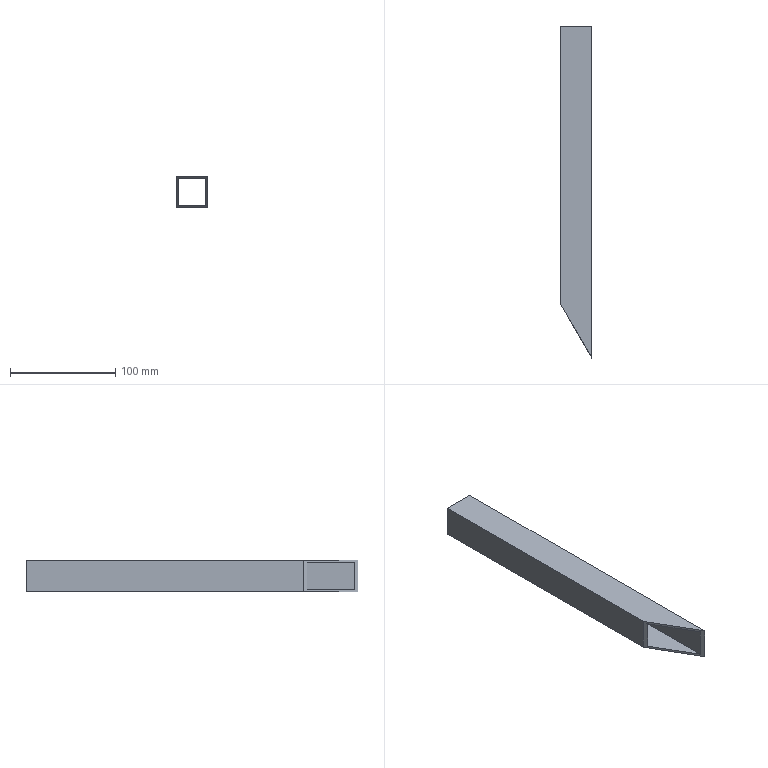Part | NX | features solid 2 | 1 solid | 10 faces | box 30 x 315 x 30 mm | volume 64740 mm3 | plane 10
STEP:
#1=CARTESIAN_POINT('',(-115.,435.,-75.));
#2=VERTEX_POINT('',#1);
#3=CARTESIAN_POINT('',(-115.,750.,-75.));
#4=VERTEX_POINT('',#3);
#5=CARTESIAN_POINT('',(-115.,615.,-75.));
#6=DIRECTION('',(0.,-1.,0.));
#7=VECTOR('',#6,1000.);
#8=LINE('',#5,#7);
#9=EDGE_CURVE('',#2,#4,#8,.F.);
#10=ORIENTED_EDGE('',*,*,#9,.F.);
#11=CARTESIAN_POINT('',(-145.,486.962,-75.));
#12=VERTEX_POINT('',#11);
#13=CARTESIAN_POINT('',(-196.692,576.495,-75.));
#14=DIRECTION('',(0.5,-0.866,0.));
#15=VECTOR('',#14,1000.);
#16=LINE('',#13,#15);
#17=EDGE_CURVE('',#2,#12,#16,.F.);
#18=ORIENTED_EDGE('',*,*,#17,.T.);
#19=CARTESIAN_POINT('',(-145.,750.,-75.));
#20=VERTEX_POINT('',#19);
#21=CARTESIAN_POINT('',(-145.,615.,-75.));
#22=DIRECTION('',(0.,-1.,0.));
#23=VECTOR('',#22,1000.);
#24=LINE('',#21,#23);
#25=EDGE_CURVE('',#12,#20,#24,.F.);
#26=ORIENTED_EDGE('',*,*,#25,.T.);
#27=CARTESIAN_POINT('',(-130.,750.,-75.));
#28=DIRECTION('',(-1.,0.,0.));
#29=VECTOR('',#28,1000.);
#30=LINE('',#27,#29);
#31=EDGE_CURVE('',#20,#4,#30,.F.);
#32=ORIENTED_EDGE('',*,*,#31,.T.);
#33=EDGE_LOOP('',(#10,#18,#26,#32));
#34=FACE_BOUND('',#33,.T.);
#35=CARTESIAN_POINT('',(-130.,615.,-75.));
#36=DIRECTION('',(0.,0.,1.));
#37=DIRECTION('',(0.,1.,0.));
#38=AXIS2_PLACEMENT_3D('',#35,#36,#37);
#39=PLANE('',#38);
#40=ADVANCED_FACE('',(#34),#39,.F.);
#41=CARTESIAN_POINT('',(-115.,435.,-45.));
#42=VERTEX_POINT('',#41);
#43=CARTESIAN_POINT('',(-145.,486.962,-45.));
#44=VERTEX_POINT('',#43);
#45=CARTESIAN_POINT('',(-196.692,576.495,-45.));
#46=DIRECTION('',(0.5,-0.866,0.));
#47=VECTOR('',#46,1000.);
#48=LINE('',#45,#47);
#49=EDGE_CURVE('',#42,#44,#48,.F.);
#50=ORIENTED_EDGE('',*,*,#49,.F.);
#51=CARTESIAN_POINT('',(-115.,750.,-45.));
#52=VERTEX_POINT('',#51);
#53=CARTESIAN_POINT('',(-115.,615.,-45.));
#54=DIRECTION('',(0.,-1.,0.));
#55=VECTOR('',#54,1000.);
#56=LINE('',#53,#55);
#57=EDGE_CURVE('',#42,#52,#56,.F.);
#58=ORIENTED_EDGE('',*,*,#57,.T.);
#59=CARTESIAN_POINT('',(-145.,750.,-45.));
#60=VERTEX_POINT('',#59);
#61=CARTESIAN_POINT('',(-130.,750.,-45.));
#62=DIRECTION('',(-1.,0.,0.));
#63=VECTOR('',#62,1000.);
#64=LINE('',#61,#63);
#65=EDGE_CURVE('',#60,#52,#64,.F.);
#66=ORIENTED_EDGE('',*,*,#65,.F.);
#67=CARTESIAN_POINT('',(-145.,615.,-45.));
#68=DIRECTION('',(0.,-1.,0.));
#69=VECTOR('',#68,1000.);
#70=LINE('',#67,#69);
#71=EDGE_CURVE('',#44,#60,#70,.F.);
#72=ORIENTED_EDGE('',*,*,#71,.F.);
#73=EDGE_LOOP('',(#50,#58,#66,#72));
#74=FACE_BOUND('',#73,.T.);
#75=CARTESIAN_POINT('',(-130.,615.,-45.));
#76=DIRECTION('',(0.,0.,1.));
#77=DIRECTION('',(0.,1.,0.));
#78=AXIS2_PLACEMENT_3D('',#75,#76,#77);
#79=PLANE('',#78);
#80=ADVANCED_FACE('',(#74),#79,.T.);
#81=ORIENTED_EDGE('',*,*,#57,.F.);
#82=CARTESIAN_POINT('',(-115.,435.,-75.));
#83=DIRECTION('',(0.,0.,-1.));
#84=VECTOR('',#83,1000.);
#85=LINE('',#82,#84);
#86=EDGE_CURVE('',#42,#2,#85,.T.);
#87=ORIENTED_EDGE('',*,*,#86,.T.);
#88=ORIENTED_EDGE('',*,*,#9,.T.);
#89=CARTESIAN_POINT('',(-115.,750.,-75.));
#90=DIRECTION('',(0.,0.,1.));
#91=VECTOR('',#90,1000.);
#92=LINE('',#89,#91);
#93=EDGE_CURVE('',#4,#52,#92,.T.);
#94=ORIENTED_EDGE('',*,*,#93,.T.);
#95=EDGE_LOOP('',(#81,#87,#88,#94));
#96=FACE_BOUND('',#95,.T.);
#97=CARTESIAN_POINT('',(-115.,615.,-75.));
#98=DIRECTION('',(1.,0.,0.));
#99=DIRECTION('',(0.,0.,-1.));
#100=AXIS2_PLACEMENT_3D('',#97,#98,#99);
#101=PLANE('',#100);
#102=ADVANCED_FACE('',(#96),#101,.T.);
#103=CARTESIAN_POINT('',(-145.,486.962,-75.));
#104=DIRECTION('',(0.,0.,-1.));
#105=VECTOR('',#104,1000.);
#106=LINE('',#103,#105);
#107=EDGE_CURVE('',#44,#12,#106,.T.);
#108=ORIENTED_EDGE('',*,*,#107,.F.);
#109=ORIENTED_EDGE('',*,*,#71,.T.);
#110=CARTESIAN_POINT('',(-145.,750.,-75.));
#111=DIRECTION('',(0.,0.,1.));
#112=VECTOR('',#111,1000.);
#113=LINE('',#110,#112);
#114=EDGE_CURVE('',#20,#60,#113,.T.);
#115=ORIENTED_EDGE('',*,*,#114,.F.);
#116=ORIENTED_EDGE('',*,*,#25,.F.);
#117=EDGE_LOOP('',(#108,#109,#115,#116));
#118=FACE_BOUND('',#117,.T.);
#119=CARTESIAN_POINT('',(-145.,615.,-75.));
#120=DIRECTION('',(1.,0.,0.));
#121=DIRECTION('',(0.,0.,-1.));
#122=AXIS2_PLACEMENT_3D('',#119,#120,#121);
#123=PLANE('',#122);
#124=ADVANCED_FACE('',(#118),#123,.F.);
#125=ORIENTED_EDGE('',*,*,#65,.T.);
#126=ORIENTED_EDGE('',*,*,#93,.F.);
#127=ORIENTED_EDGE('',*,*,#31,.F.);
#128=ORIENTED_EDGE('',*,*,#114,.T.);
#129=EDGE_LOOP('',(#125,#126,#127,#128));
#130=FACE_BOUND('',#129,.T.);
#131=CARTESIAN_POINT('',(-143.,750.,-47.));
#132=VERTEX_POINT('',#131);
#133=CARTESIAN_POINT('',(-117.,750.,-47.));
#134=VERTEX_POINT('',#133);
#135=CARTESIAN_POINT('',(-130.,750.,-47.));
#136=DIRECTION('',(-1.,0.,0.));
#137=VECTOR('',#136,1000.);
#138=LINE('',#135,#137);
#139=EDGE_CURVE('',#132,#134,#138,.F.);
#140=ORIENTED_EDGE('',*,*,#139,.F.);
#141=CARTESIAN_POINT('',(-143.,750.,-73.));
#142=VERTEX_POINT('',#141);
#143=CARTESIAN_POINT('',(-143.,750.,-75.));
#144=DIRECTION('',(0.,0.,1.));
#145=VECTOR('',#144,1000.);
#146=LINE('',#143,#145);
#147=EDGE_CURVE('',#142,#132,#146,.T.);
#148=ORIENTED_EDGE('',*,*,#147,.F.);
#149=CARTESIAN_POINT('',(-117.,750.,-73.));
#150=VERTEX_POINT('',#149);
#151=CARTESIAN_POINT('',(-130.,750.,-73.));
#152=DIRECTION('',(-1.,0.,0.));
#153=VECTOR('',#152,1000.);
#154=LINE('',#151,#153);
#155=EDGE_CURVE('',#142,#150,#154,.F.);
#156=ORIENTED_EDGE('',*,*,#155,.T.);
#157=CARTESIAN_POINT('',(-117.,750.,-75.));
#158=DIRECTION('',(0.,0.,1.));
#159=VECTOR('',#158,1000.);
#160=LINE('',#157,#159);
#161=EDGE_CURVE('',#150,#134,#160,.T.);
#162=ORIENTED_EDGE('',*,*,#161,.T.);
#163=EDGE_LOOP('',(#140,#148,#156,#162));
#164=FACE_BOUND('',#163,.T.);
#165=CARTESIAN_POINT('',(-130.,750.,-75.));
#166=DIRECTION('',(0.,-1.,0.));
#167=DIRECTION('',(0.,0.,-1.));
#168=AXIS2_PLACEMENT_3D('',#165,#166,#167);
#169=PLANE('',#168);
#170=ADVANCED_FACE('',(#130,#164),#169,.F.);
#171=CARTESIAN_POINT('',(-117.,438.464,-73.));
#172=VERTEX_POINT('',#171);
#173=CARTESIAN_POINT('',(-143.,483.497,-73.));
#174=VERTEX_POINT('',#173);
#175=CARTESIAN_POINT('',(-196.692,576.495,-73.));
#176=DIRECTION('',(0.5,-0.866,0.));
#177=VECTOR('',#176,1000.);
#178=LINE('',#175,#177);
#179=EDGE_CURVE('',#172,#174,#178,.F.);
#180=ORIENTED_EDGE('',*,*,#179,.F.);
#181=CARTESIAN_POINT('',(-117.,615.,-73.));
#182=DIRECTION('',(0.,-1.,0.));
#183=VECTOR('',#182,1000.);
#184=LINE('',#181,#183);
#185=EDGE_CURVE('',#172,#150,#184,.F.);
#186=ORIENTED_EDGE('',*,*,#185,.T.);
#187=ORIENTED_EDGE('',*,*,#155,.F.);
#188=CARTESIAN_POINT('',(-143.,615.,-73.));
#189=DIRECTION('',(0.,-1.,0.));
#190=VECTOR('',#189,1000.);
#191=LINE('',#188,#190);
#192=EDGE_CURVE('',#174,#142,#191,.F.);
#193=ORIENTED_EDGE('',*,*,#192,.F.);
#194=EDGE_LOOP('',(#180,#186,#187,#193));
#195=FACE_BOUND('',#194,.T.);
#196=CARTESIAN_POINT('',(-130.,615.,-73.));
#197=DIRECTION('',(0.,0.,1.));
#198=DIRECTION('',(0.,1.,0.));
#199=AXIS2_PLACEMENT_3D('',#196,#197,#198);
#200=PLANE('',#199);
#201=ADVANCED_FACE('',(#195),#200,.T.);
#202=CARTESIAN_POINT('',(-117.,438.464,-47.));
#203=VERTEX_POINT('',#202);
#204=CARTESIAN_POINT('',(-117.,615.,-47.));
#205=DIRECTION('',(0.,-1.,0.));
#206=VECTOR('',#205,1000.);
#207=LINE('',#204,#206);
#208=EDGE_CURVE('',#203,#134,#207,.F.);
#209=ORIENTED_EDGE('',*,*,#208,.F.);
#210=CARTESIAN_POINT('',(-143.,483.497,-47.));
#211=VERTEX_POINT('',#210);
#212=CARTESIAN_POINT('',(-196.692,576.495,-47.));
#213=DIRECTION('',(0.5,-0.866,0.));
#214=VECTOR('',#213,1000.);
#215=LINE('',#212,#214);
#216=EDGE_CURVE('',#203,#211,#215,.F.);
#217=ORIENTED_EDGE('',*,*,#216,.T.);
#218=CARTESIAN_POINT('',(-143.,615.,-47.));
#219=DIRECTION('',(0.,-1.,0.));
#220=VECTOR('',#219,1000.);
#221=LINE('',#218,#220);
#222=EDGE_CURVE('',#211,#132,#221,.F.);
#223=ORIENTED_EDGE('',*,*,#222,.T.);
#224=ORIENTED_EDGE('',*,*,#139,.T.);
#225=EDGE_LOOP('',(#209,#217,#223,#224));
#226=FACE_BOUND('',#225,.T.);
#227=CARTESIAN_POINT('',(-130.,615.,-47.));
#228=DIRECTION('',(0.,0.,1.));
#229=DIRECTION('',(0.,1.,0.));
#230=AXIS2_PLACEMENT_3D('',#227,#228,#229);
#231=PLANE('',#230);
#232=ADVANCED_FACE('',(#226),#231,.F.);
#233=CARTESIAN_POINT('',(-117.,438.464,-75.));
#234=DIRECTION('',(0.,0.,-1.));
#235=VECTOR('',#234,1000.);
#236=LINE('',#233,#235);
#237=EDGE_CURVE('',#203,#172,#236,.T.);
#238=ORIENTED_EDGE('',*,*,#237,.F.);
#239=ORIENTED_EDGE('',*,*,#208,.T.);
#240=ORIENTED_EDGE('',*,*,#161,.F.);
#241=ORIENTED_EDGE('',*,*,#185,.F.);
#242=EDGE_LOOP('',(#238,#239,#240,#241));
#243=FACE_BOUND('',#242,.T.);
#244=CARTESIAN_POINT('',(-117.,615.,-75.));
#245=DIRECTION('',(1.,0.,0.));
#246=DIRECTION('',(0.,0.,-1.));
#247=AXIS2_PLACEMENT_3D('',#244,#245,#246);
#248=PLANE('',#247);
#249=ADVANCED_FACE('',(#243),#248,.F.);
#250=ORIENTED_EDGE('',*,*,#222,.F.);
#251=CARTESIAN_POINT('',(-143.,483.497,-75.));
#252=DIRECTION('',(0.,0.,-1.));
#253=VECTOR('',#252,1000.);
#254=LINE('',#251,#253);
#255=EDGE_CURVE('',#211,#174,#254,.T.);
#256=ORIENTED_EDGE('',*,*,#255,.T.);
#257=ORIENTED_EDGE('',*,*,#192,.T.);
#258=ORIENTED_EDGE('',*,*,#147,.T.);
#259=EDGE_LOOP('',(#250,#256,#257,#258));
#260=FACE_BOUND('',#259,.T.);
#261=CARTESIAN_POINT('',(-143.,615.,-75.));
#262=DIRECTION('',(1.,0.,0.));
#263=DIRECTION('',(0.,0.,-1.));
#264=AXIS2_PLACEMENT_3D('',#261,#262,#263);
#265=PLANE('',#264);
#266=ADVANCED_FACE('',(#260),#265,.T.);
#267=ORIENTED_EDGE('',*,*,#17,.F.);
#268=ORIENTED_EDGE('',*,*,#86,.F.);
#269=ORIENTED_EDGE('',*,*,#49,.T.);
#270=ORIENTED_EDGE('',*,*,#107,.T.);
#271=EDGE_LOOP('',(#267,#268,#269,#270));
#272=FACE_BOUND('',#271,.T.);
#273=ORIENTED_EDGE('',*,*,#237,.T.);
#274=ORIENTED_EDGE('',*,*,#179,.T.);
#275=ORIENTED_EDGE('',*,*,#255,.F.);
#276=ORIENTED_EDGE('',*,*,#216,.F.);
#277=EDGE_LOOP('',(#273,#274,#275,#276));
#278=FACE_BOUND('',#277,.T.);
#279=CARTESIAN_POINT('',(-115.,435.,-45.));
#280=DIRECTION('',(-0.866,-0.5,0.));
#281=DIRECTION('',(0.5,-0.866,0.));
#282=AXIS2_PLACEMENT_3D('',#279,#280,#281);
#283=PLANE('',#282);
#284=ADVANCED_FACE('',(#272,#278),#283,.T.);
#285=CLOSED_SHELL('',(#40,#80,#102,#124,#170,#201,#232,#249,#266,#284));
#286=MANIFOLD_SOLID_BREP('',#285);
#287=(LENGTH_UNIT()NAMED_UNIT(*)SI_UNIT(.MILLI.,.METRE.));
#288=UNCERTAINTY_MEASURE_WITH_UNIT(LENGTH_MEASURE(0.00001),#287,'','');
#289=(NAMED_UNIT(*)PLANE_ANGLE_UNIT()SI_UNIT($,.RADIAN.));
#290=(NAMED_UNIT(*)SI_UNIT($,.STERADIAN.)SOLID_ANGLE_UNIT());
#291=(GEOMETRIC_REPRESENTATION_CONTEXT(3)GLOBAL_UNCERTAINTY_ASSIGNED_CONTEXT((#288))GLOBAL_UNIT_ASSIGNED_CONTEXT((#287,#289,#290))REPRESENTATION_CONTEXT('',''));
#292=ADVANCED_BREP_SHAPE_REPRESENTATION('',(#286),#291);